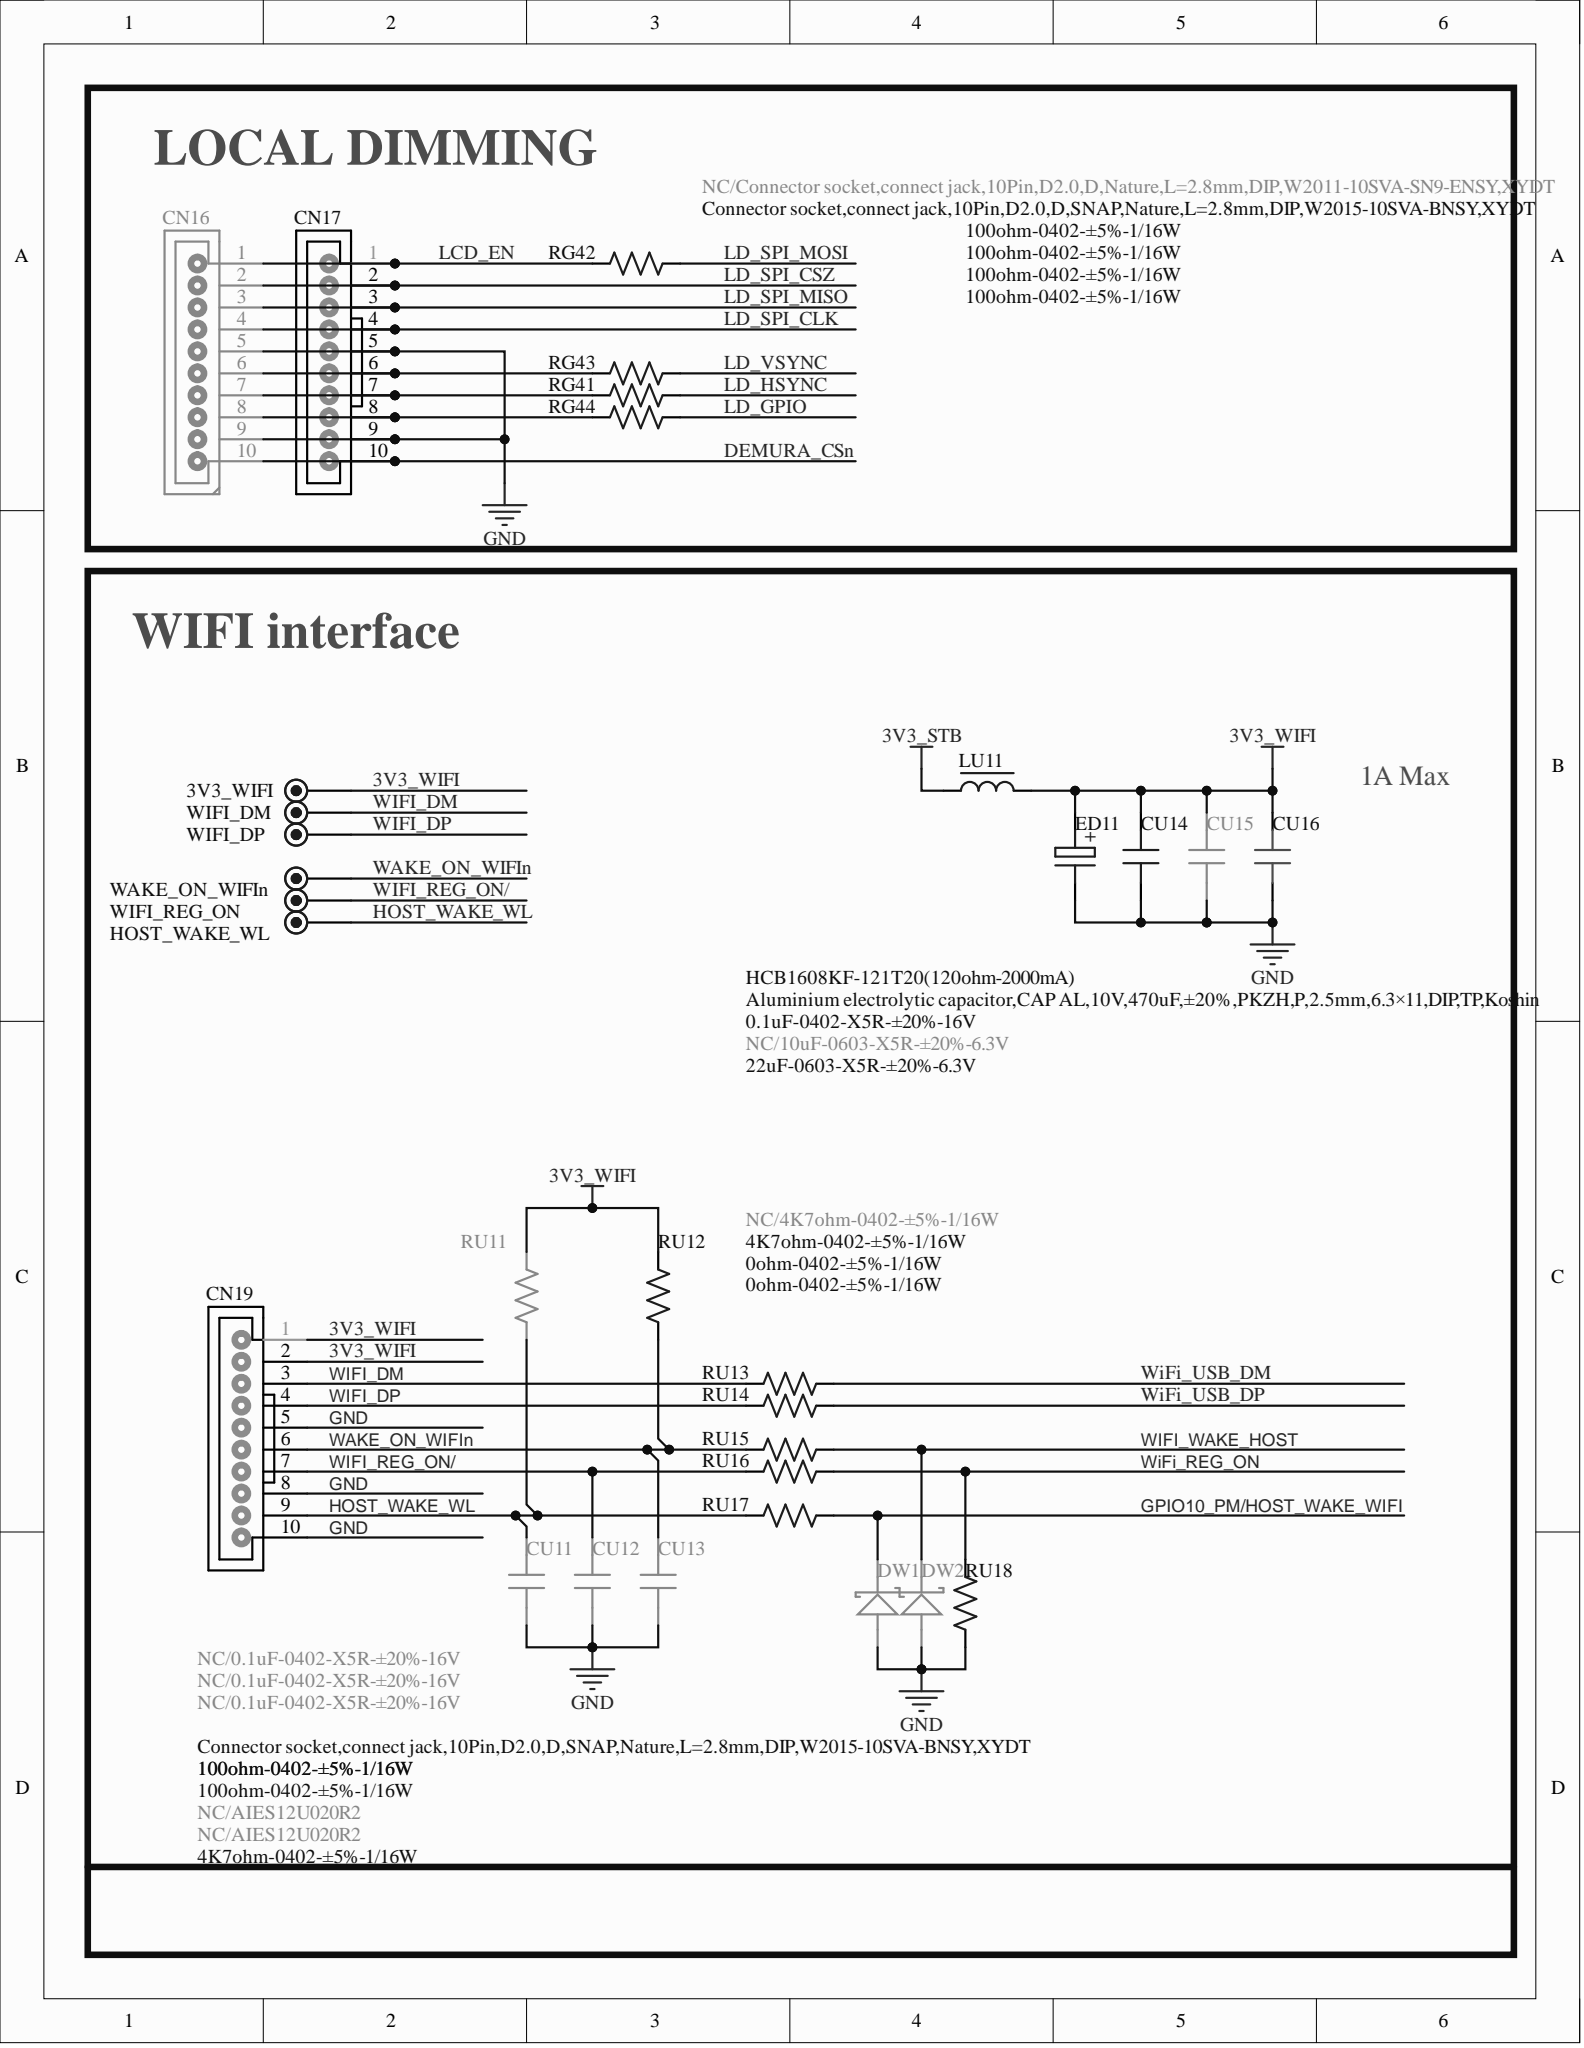Circuit board | Altium Designer | 1029 parts | 642 nets | one sheet of the schematic
Parts on this sheet (reference | value | footprint):
CN16 | NC/Connector socket,connect jack,10Pin,D2.0,D,Nature,L=2.8mm,DIP,W2011-10SVA-SN9-ENSY,XYDT | SIP10/2.0D-1
CN17 | Connector socket,connect jack,10Pin,D2.0,D,SNAP,Nature,L=2.8mm,DIP,W2015-10SVA-BNSY,XYDT | SIP10/2.0D-4
CN19 | Connector socket,connect jack,10Pin,D2.0,D,SNAP,Nature,L=2.8mm,DIP,W2015-10SVA-BNSY,XYDT | SIP10/2.0D-4
CU11 | NC/0.1uF-0402-X5R-±20%-16V | C0402
CU12 | NC/0.1uF-0402-X5R-±20%-16V | C0402
CU13 | NC/0.1uF-0402-X5R-±20%-16V | C0402
CU14 | 0.1uF-0402-X5R-±20%-16V | C0402
CU15 | NC/10uF-0603-X5R-±20%-6.3V | C0603
CU16 | 22uF-0603-X5R-±20%-6.3V | C0603
DW1 | NC/AIES12U020R2 | DIODE-S0402
DW2 | NC/AIES12U020R2 | DIODE-S0402
HOST_WAKE_WL | TEST | TP
LU11 | HCB1608KF-121T20(120ohm-2000mA) | L0603
RG41 | 100ohm-0402-±5%-1/16W | R0402
RG42 | 100ohm-0402-±5%-1/16W | R0402
RG43 | 100ohm-0402-±5%-1/16W | R0402
RG44 | 100ohm-0402-±5%-1/16W | R0402
RU11 | NC/4K7ohm-0402-±5%-1/16W | R0402
RU12 | 4K7ohm-0402-±5%-1/16W | R0402
RU13 | 0ohm-0402-±5%-1/16W | R0402
RU14 | 0ohm-0402-±5%-1/16W | R0402
RU15 | 100ohm-0402-±5%-1/16W | R0402
RU16 | 100ohm-0402-±5%-1/16W | R0402
RU17 | 100ohm-0402-±5%-1/16W | R0402
RU18 | 4K7ohm-0402-±5%-1/16W | R0402
WAKE_ON_WIFIn | TEST | TP
WIFI_DM | TEST | TP
WIFI_DP | TEST | TP
WIFI_REG_ON | TEST | TP
Nets of these parts (net: part-pin ...):
WIFI_WAKE_HOST: DW2-K RU15-2
WiFi_USB_DP: RU14-2
WiFi_USB_DM: RU13-2
WIFI_REG_ON/: CN19-7 CU12-1 RU16-1 WIFI_REG_ON-1
WiFi_REG_ON: RU16-2 RU18-2
WIFI_DP: CN19-4 RU14-1 WIFI_DP-1
WIFI_DM: CN19-3 RU13-1 WIFI_DM-1
WAKE_ON_WIFIn: CN19-6 CU13-1 RU12-1 RU15-1 WAKE_ON_WIFIn-1
NetCN16_8: CN16-8 CN17-8 RG44-1
NetCN16_7: CN16-7 CN17-7 RG41-1
NetCN16_6: CN16-6 CN17-6 RG43-1
LD_VSYNC: RG43-2
LD_SPI_MOSI: RG42-2
LD_SPI_MISO: CN16-3 CN17-3
LD_SPI_CSZ: CN16-2 CN17-2
LD_SPI_CLK: CN16-4 CN17-4
LD_HSYNC: RG41-2
LD_GPIO: RG44-2
LCD_EN: CN16-1 CN17-1 RG42-1
HOST_WAKE_WL: CN19-9 CU11-1 HOST_WAKE_WL-1 RU11-1 RU17-1
GPIO10_PM/HOST_WAKE_WIFI: DW1-K RU17-2
GND: CN16-5 CN16-9 CN17-5 CN17-9 CN19-5 CN19-8 CN19-10 CU11-2 CU12-2 CU13-2 CU14-1 CU15-1 CU16-1 DW1-A DW2-A RU18-1
DEMURA_CSn: CN16-10 CN17-10
3V3_WIFI: CN19-1 CN19-2 CU14-2 CU15-2 CU16-2 LU11-2 RU11-2 RU12-2
3V3_STB: LU11-1